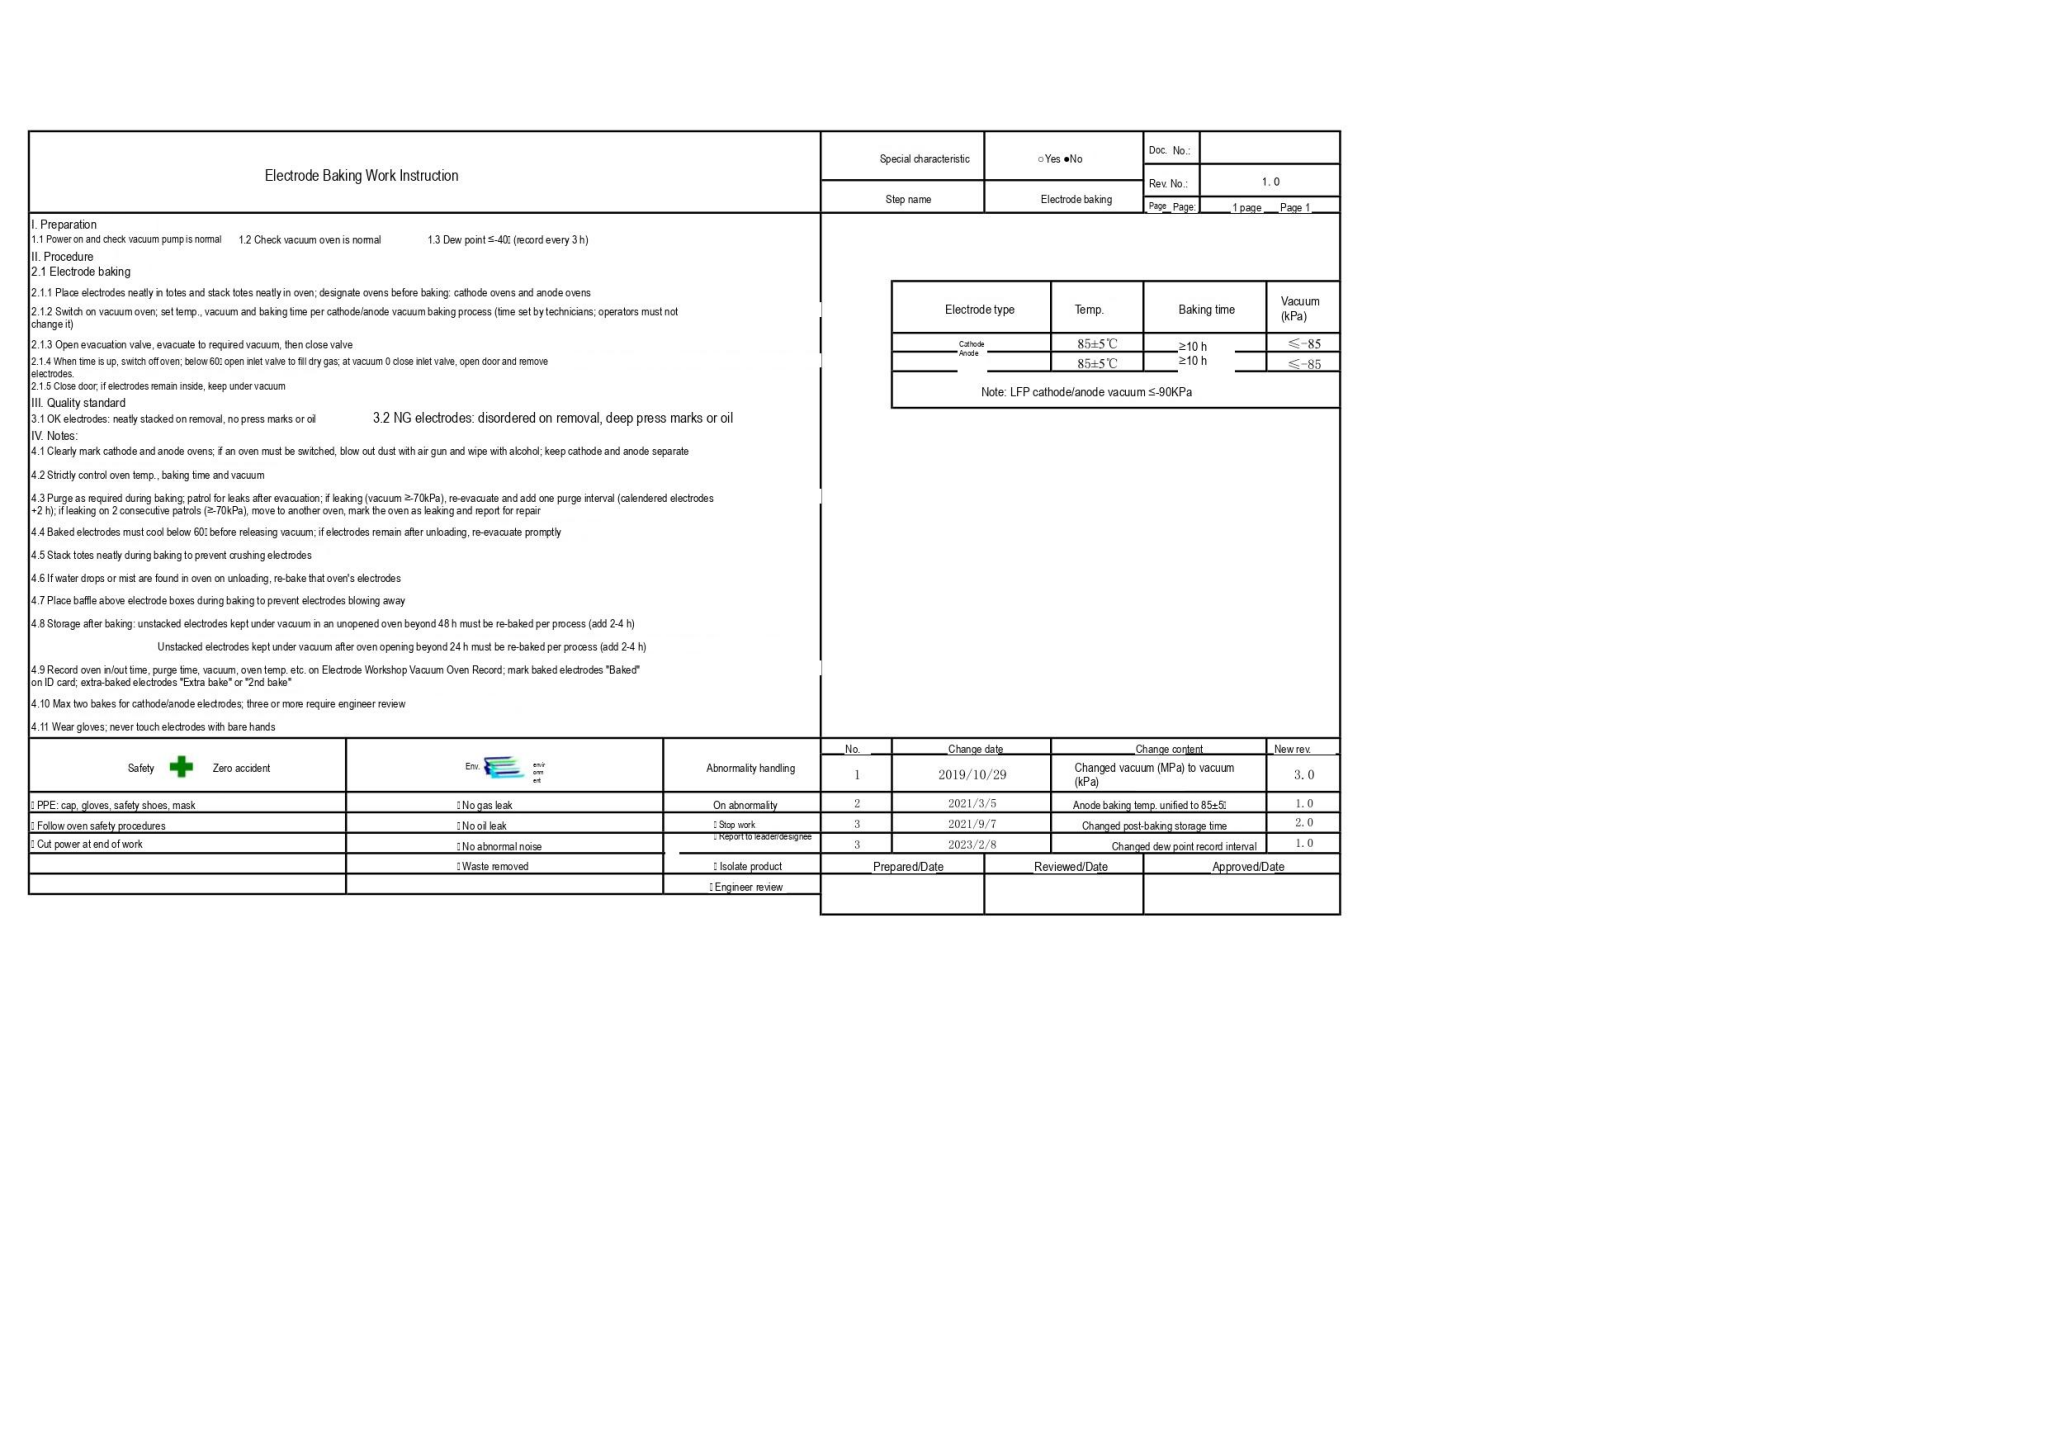# Electrode Baking Work Instruction

| Special characteristic | ○Yes ●No | Doc. No.: | |
|---|---|---|---|
| Step name | Electrode baking | Rev. No.: | 1.0 |
| | | Page Page: | 1 page Page 1 |

I. Preparation
1.1 Power on and check vacuum pump is normal 1.2 Check vacuum oven is normal 1.3 Dew point ≤-40 (record every 3 h)
II. Procedure
2.1 Electrode baking
2.1.1 Place electrodes neatly in totes and stack totes neatly in oven; designate ovens before baking: cathode ovens and anode ovens
2.1.2 Switch on vacuum oven; set temp., vacuum and baking time per cathode/anode vacuum baking process (time set by technicians; operators must not change it)
2.1.3 Open evacuation valve, evacuate to required vacuum, then close valve
2.1.4 When time is up, switch off oven; below 60 open inlet valve to fill dry gas; at vacuum 0 close inlet valve, open door and remove electrodes.
2.1.5 Close door; if electrodes remain inside, keep under vacuum
III. Quality standard
3.1 OK electrodes: neatly stacked on removal, no press marks or oil 3.2 NG electrodes: disordered on removal, deep press marks or oil
IV. Notes:
4.1 Clearly mark cathode and anode ovens; if an oven must be switched, blow out dust with air gun and wipe with alcohol; keep cathode and anode separate
4.2 Strictly control oven temp., baking time and vacuum
4.3 Purge as required during baking; patrol for leaks after evacuation; if leaking (vacuum ≥-70kPa), re-evacuate and add one purge interval (calendered electrodes +2 h); if leaking on 2 consecutive patrols (≥-70kPa), move to another oven, mark the oven as leaking and report for repair
4.4 Baked electrodes must cool below 60 before releasing vacuum; if electrodes remain after unloading, re-evacuate promptly
4.5 Stack totes neatly during baking to prevent crushing electrodes
4.6 If water drops or mist are found in oven on unloading, re-bake that oven's electrodes
4.7 Place baffle above electrode boxes during baking to prevent electrodes blowing away
4.8 Storage after baking: unstacked electrodes kept under vacuum in an unopened oven beyond 48 h must be re-baked per process (add 2-4 h)
Unstacked electrodes kept under vacuum after oven opening beyond 24 h must be re-baked per process (add 2-4 h)
4.9 Record oven in/out time, purge time, vacuum, oven temp. etc. on Electrode Workshop Vacuum Oven Record; mark baked electrodes "Baked" on ID card; extra-baked electrodes "Extra bake" or "2nd bake"
4.10 Max two bakes for cathode/anode electrodes; three or more require engineer review
4.11 Wear gloves; never touch electrodes with bare hands

| Electrode type | Temp. | Baking time | Vacuum (kPa) |
|---|---|---|---|
| Cathode | 85±5℃ | ≥10 h | ≤-85 |
| Anode | 85±5℃ | ≥10 h | ≤-85 |

Note: LFP cathode/anode vacuum ≤-90KPa

| Safety Zero accident | Env. envir onm ent | Abnormality handling |
|---|---|---|
| PPE: cap, gloves, safety shoes, mask | No gas leak | On abnormality |
| Follow oven safety procedures | No oil leak | Stop work |
| Cut power at end of work | No abnormal noise | Report to leader/designee |
| | Waste removed | Isolate product |
| | | Engineer review |

| No. | Change date | Change content | New rev. |
|---|---|---|---|
| 1 | 2019/10/29 | Changed vacuum (MPa) to vacuum (kPa) | 3.0 |
| 2 | 2021/3/5 | Anode baking temp. unified to 85±5 | 1.0 |
| 3 | 2021/9/7 | Changed post-baking storage time | 2.0 |
| 3 | 2023/2/8 | Changed dew point record interval | 1.0 |

| Prepared/Date | Reviewed/Date | Approved/Date |
|---|---|---|
| | | |